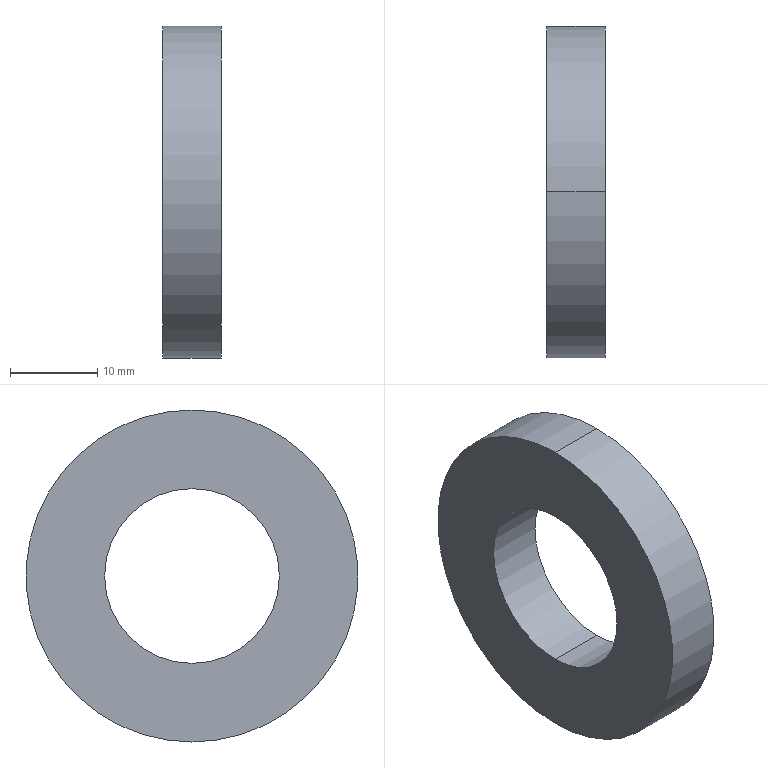Part | SolidWorks | features Extrusion 1 | 1 solid | 6 faces | box 6.7 x 38 x 38 mm | volume 5494 mm3 | cylinder 4 | plane 2 | commonest cylinder face diameters 20 x2 38 x2
STEP:
#1=CARTESIAN_POINT('',(6.7,0.,10.));
#2=VERTEX_POINT('',#1);
#3=CARTESIAN_POINT('',(6.7,0.,-10.));
#4=VERTEX_POINT('',#3);
#5=CARTESIAN_POINT('',(6.7,0.,0.));
#6=DIRECTION('',(1.,0.,0.));
#7=DIRECTION('',(0.,0.,-1.));
#8=AXIS2_PLACEMENT_3D('',#5,#6,#7);
#9=CIRCLE('',#8,10.);
#10=EDGE_CURVE('',#2,#4,#9,.T.);
#11=ORIENTED_EDGE('',*,*,#10,.T.);
#12=CARTESIAN_POINT('',(0.,0.,-10.));
#13=VERTEX_POINT('',#12);
#14=CARTESIAN_POINT('',(6.7,0.,-10.));
#15=DIRECTION('',(-1.,0.,0.));
#16=VECTOR('',#15,1000.);
#17=LINE('',#14,#16);
#18=EDGE_CURVE('',#4,#13,#17,.T.);
#19=ORIENTED_EDGE('',*,*,#18,.T.);
#20=CARTESIAN_POINT('',(0.,0.,10.));
#21=VERTEX_POINT('',#20);
#22=CARTESIAN_POINT('',(0.,0.,0.));
#23=DIRECTION('',(1.,0.,0.));
#24=DIRECTION('',(0.,0.,-1.));
#25=AXIS2_PLACEMENT_3D('',#22,#23,#24);
#26=CIRCLE('',#25,10.);
#27=EDGE_CURVE('',#21,#13,#26,.T.);
#28=ORIENTED_EDGE('',*,*,#27,.F.);
#29=CARTESIAN_POINT('',(6.7,0.,10.));
#30=DIRECTION('',(-1.,0.,0.));
#31=VECTOR('',#30,1000.);
#32=LINE('',#29,#31);
#33=EDGE_CURVE('',#2,#21,#32,.T.);
#34=ORIENTED_EDGE('',*,*,#33,.F.);
#35=EDGE_LOOP('',(#11,#19,#28,#34));
#36=FACE_OUTER_BOUND('',#35,.T.);
#37=CARTESIAN_POINT('',(6.7,0.,0.));
#38=DIRECTION('',(-1.,0.,0.));
#39=DIRECTION('',(0.,0.,1.));
#40=AXIS2_PLACEMENT_3D('',#37,#38,#39);
#41=CYLINDRICAL_SURFACE('',#40,10.);
#42=ADVANCED_FACE('',(#36),#41,.F.);
#43=CARTESIAN_POINT('',(6.7,0.,-19.));
#44=VERTEX_POINT('',#43);
#45=CARTESIAN_POINT('',(6.7,0.,19.));
#46=VERTEX_POINT('',#45);
#47=CARTESIAN_POINT('',(6.7,0.,0.));
#48=DIRECTION('',(1.,0.,0.));
#49=DIRECTION('',(0.,0.,-1.));
#50=AXIS2_PLACEMENT_3D('',#47,#48,#49);
#51=CIRCLE('',#50,19.);
#52=EDGE_CURVE('',#44,#46,#51,.T.);
#53=ORIENTED_EDGE('',*,*,#52,.F.);
#54=CARTESIAN_POINT('',(0.,0.,-19.));
#55=VERTEX_POINT('',#54);
#56=CARTESIAN_POINT('',(6.7,0.,-19.));
#57=DIRECTION('',(-1.,0.,0.));
#58=VECTOR('',#57,1000.);
#59=LINE('',#56,#58);
#60=EDGE_CURVE('',#44,#55,#59,.T.);
#61=ORIENTED_EDGE('',*,*,#60,.T.);
#62=CARTESIAN_POINT('',(0.,0.,19.));
#63=VERTEX_POINT('',#62);
#64=CARTESIAN_POINT('',(0.,0.,0.));
#65=DIRECTION('',(1.,0.,0.));
#66=DIRECTION('',(0.,0.,-1.));
#67=AXIS2_PLACEMENT_3D('',#64,#65,#66);
#68=CIRCLE('',#67,19.);
#69=EDGE_CURVE('',#55,#63,#68,.T.);
#70=ORIENTED_EDGE('',*,*,#69,.T.);
#71=CARTESIAN_POINT('',(6.7,0.,19.));
#72=DIRECTION('',(-1.,0.,0.));
#73=VECTOR('',#72,1000.);
#74=LINE('',#71,#73);
#75=EDGE_CURVE('',#46,#63,#74,.T.);
#76=ORIENTED_EDGE('',*,*,#75,.F.);
#77=EDGE_LOOP('',(#53,#61,#70,#76));
#78=FACE_OUTER_BOUND('',#77,.T.);
#79=CARTESIAN_POINT('',(6.7,0.,0.));
#80=DIRECTION('',(-1.,0.,0.));
#81=DIRECTION('',(0.,0.,1.));
#82=AXIS2_PLACEMENT_3D('',#79,#80,#81);
#83=CYLINDRICAL_SURFACE('',#82,19.);
#84=ADVANCED_FACE('',(#78),#83,.T.);
#85=CARTESIAN_POINT('',(6.7,0.,0.));
#86=DIRECTION('',(1.,0.,0.));
#87=DIRECTION('',(0.,0.,-1.));
#88=AXIS2_PLACEMENT_3D('',#85,#86,#87);
#89=CIRCLE('',#88,19.);
#90=EDGE_CURVE('',#46,#44,#89,.T.);
#91=ORIENTED_EDGE('',*,*,#90,.T.);
#92=ORIENTED_EDGE('',*,*,#52,.T.);
#93=EDGE_LOOP('',(#91,#92));
#94=FACE_OUTER_BOUND('',#93,.T.);
#95=ORIENTED_EDGE('',*,*,#10,.F.);
#96=CARTESIAN_POINT('',(6.7,0.,0.));
#97=DIRECTION('',(1.,0.,0.));
#98=DIRECTION('',(0.,0.,-1.));
#99=AXIS2_PLACEMENT_3D('',#96,#97,#98);
#100=CIRCLE('',#99,10.);
#101=EDGE_CURVE('',#4,#2,#100,.T.);
#102=ORIENTED_EDGE('',*,*,#101,.F.);
#103=EDGE_LOOP('',(#95,#102));
#104=FACE_BOUND('',#103,.T.);
#105=CARTESIAN_POINT('',(6.7,0.,0.));
#106=DIRECTION('',(1.,0.,0.));
#107=DIRECTION('',(0.,0.,-1.));
#108=AXIS2_PLACEMENT_3D('',#105,#106,#107);
#109=PLANE('',#108);
#110=ADVANCED_FACE('',(#94,#104),#109,.T.);
#111=CARTESIAN_POINT('',(0.,0.,0.));
#112=DIRECTION('',(1.,0.,0.));
#113=DIRECTION('',(0.,0.,-1.));
#114=AXIS2_PLACEMENT_3D('',#111,#112,#113);
#115=CIRCLE('',#114,19.);
#116=EDGE_CURVE('',#63,#55,#115,.T.);
#117=ORIENTED_EDGE('',*,*,#116,.F.);
#118=ORIENTED_EDGE('',*,*,#69,.F.);
#119=EDGE_LOOP('',(#117,#118));
#120=FACE_OUTER_BOUND('',#119,.T.);
#121=ORIENTED_EDGE('',*,*,#27,.T.);
#122=CARTESIAN_POINT('',(0.,0.,0.));
#123=DIRECTION('',(1.,0.,0.));
#124=DIRECTION('',(0.,0.,-1.));
#125=AXIS2_PLACEMENT_3D('',#122,#123,#124);
#126=CIRCLE('',#125,10.);
#127=EDGE_CURVE('',#13,#21,#126,.T.);
#128=ORIENTED_EDGE('',*,*,#127,.T.);
#129=EDGE_LOOP('',(#121,#128));
#130=FACE_BOUND('',#129,.T.);
#131=CARTESIAN_POINT('',(0.,0.,0.));
#132=DIRECTION('',(1.,0.,0.));
#133=DIRECTION('',(0.,0.,-1.));
#134=AXIS2_PLACEMENT_3D('',#131,#132,#133);
#135=PLANE('',#134);
#136=ADVANCED_FACE('',(#120,#130),#135,.F.);
#137=ORIENTED_EDGE('',*,*,#60,.F.);
#138=ORIENTED_EDGE('',*,*,#90,.F.);
#139=ORIENTED_EDGE('',*,*,#75,.T.);
#140=ORIENTED_EDGE('',*,*,#116,.T.);
#141=EDGE_LOOP('',(#137,#138,#139,#140));
#142=FACE_OUTER_BOUND('',#141,.T.);
#143=CARTESIAN_POINT('',(6.7,0.,0.));
#144=DIRECTION('',(-1.,0.,0.));
#145=DIRECTION('',(0.,0.,1.));
#146=AXIS2_PLACEMENT_3D('',#143,#144,#145);
#147=CYLINDRICAL_SURFACE('',#146,19.);
#148=ADVANCED_FACE('',(#142),#147,.T.);
#149=ORIENTED_EDGE('',*,*,#18,.F.);
#150=ORIENTED_EDGE('',*,*,#101,.T.);
#151=ORIENTED_EDGE('',*,*,#33,.T.);
#152=ORIENTED_EDGE('',*,*,#127,.F.);
#153=EDGE_LOOP('',(#149,#150,#151,#152));
#154=FACE_OUTER_BOUND('',#153,.T.);
#155=CARTESIAN_POINT('',(6.7,0.,0.));
#156=DIRECTION('',(-1.,0.,0.));
#157=DIRECTION('',(0.,0.,1.));
#158=AXIS2_PLACEMENT_3D('',#155,#156,#157);
#159=CYLINDRICAL_SURFACE('',#158,10.);
#160=ADVANCED_FACE('',(#154),#159,.F.);
#161=CLOSED_SHELL('',(#42,#84,#110,#136,#148,#160));
#162=MANIFOLD_SOLID_BREP('',#161);
#163=CARTESIAN_POINT('',(0.,0.,0.));
#164=DIRECTION('',(0.,0.,1.));
#165=DIRECTION('',(1.,0.,0.));
#166=AXIS2_PLACEMENT_3D('',#163,#164,#165);
#167=(LENGTH_UNIT()NAMED_UNIT(*)SI_UNIT(.MILLI.,.METRE.));
#168=UNCERTAINTY_MEASURE_WITH_UNIT(LENGTH_MEASURE(0.00001),#167,'','');
#169=(NAMED_UNIT(*)PLANE_ANGLE_UNIT()SI_UNIT($,.RADIAN.));
#170=(NAMED_UNIT(*)SI_UNIT($,.STERADIAN.)SOLID_ANGLE_UNIT());
#171=(GEOMETRIC_REPRESENTATION_CONTEXT(3)GLOBAL_UNCERTAINTY_ASSIGNED_CONTEXT((#168))GLOBAL_UNIT_ASSIGNED_CONTEXT((#167,#169,#170))REPRESENTATION_CONTEXT('',''));
#172=ADVANCED_BREP_SHAPE_REPRESENTATION('',(#162,#166),#171);